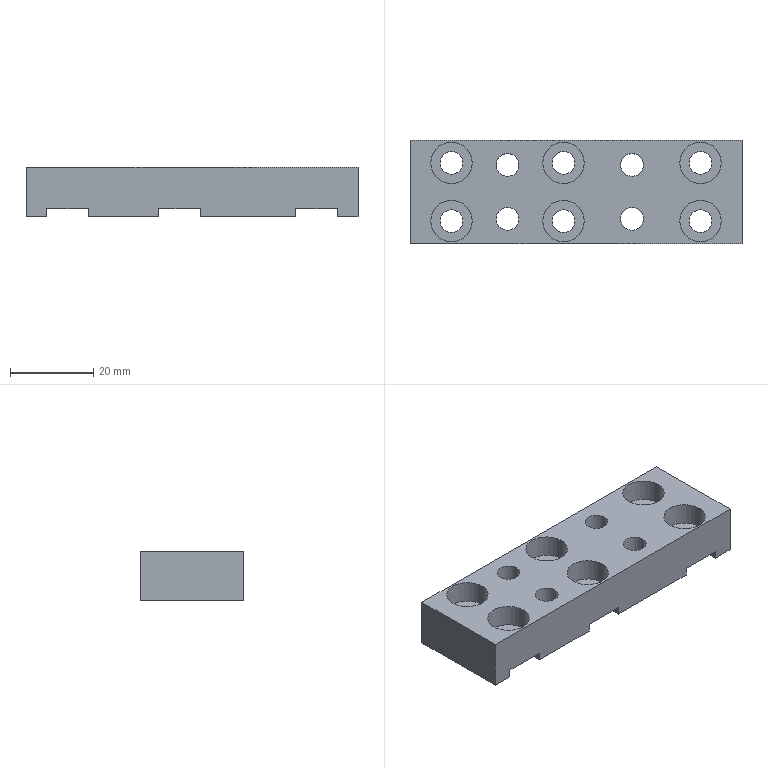Part | SolidWorks | features HoleWzd 2, Extrusion 1, ICE 1 | 1 solid | 68 faces | box 80 x 25 x 12 mm | volume 16976 mm3 | cylinder 40 | plane 28 | commonest cylinder face diameters 5.5 x20 10 x20